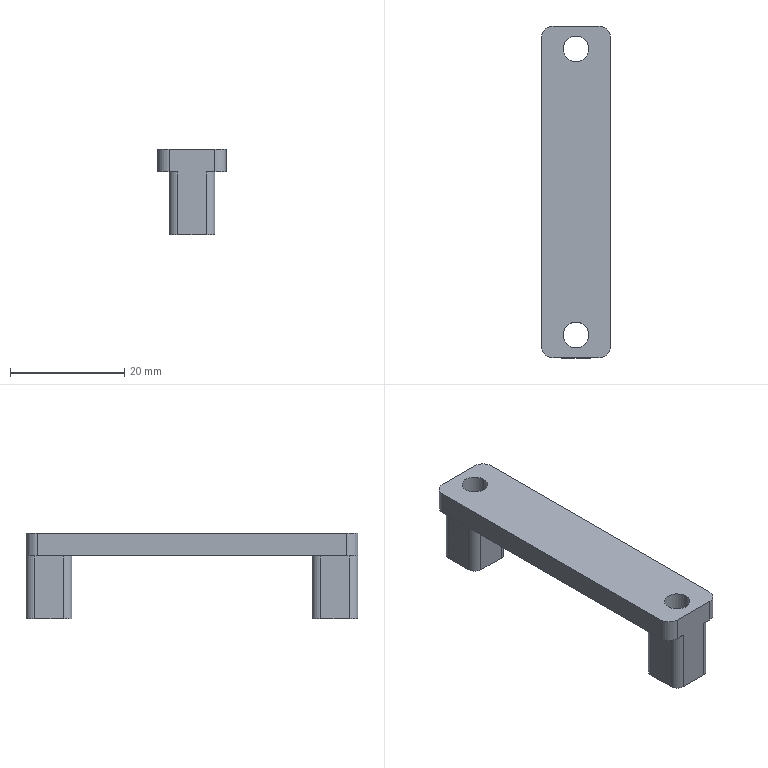Part | SolidWorks | features BaseBody 1 | 1 solid | 30 faces | box 12 x 58 x 15 mm | volume 3659 mm3 | cylinder 16 | plane 14 | commonest cylinder face diameters 3 x8 4 x4 4.5 x4
STEP:
#1=CARTESIAN_POINT('',(607.2,-29.,223.536));
#2=VERTEX_POINT('',#1);
#3=CARTESIAN_POINT('',(611.7,-29.,223.536));
#4=VERTEX_POINT('',#3);
#5=CARTESIAN_POINT('',(609.45,-29.,223.536));
#6=DIRECTION('',(0.,0.,1.));
#7=DIRECTION('',(1.,0.,0.));
#8=AXIS2_PLACEMENT_3D('',#5,#6,#7);
#9=CIRCLE('',#8,2.25);
#10=EDGE_CURVE('',#2,#4,#9,.T.);
#11=ORIENTED_EDGE('',*,*,#10,.F.);
#12=CARTESIAN_POINT('',(607.2,-29.,238.536));
#13=VERTEX_POINT('',#12);
#14=CARTESIAN_POINT('',(607.2,-29.,238.536));
#15=DIRECTION('',(0.,0.,1.));
#16=VECTOR('',#15,1000.);
#17=LINE('',#14,#16);
#18=EDGE_CURVE('',#2,#13,#17,.T.);
#19=ORIENTED_EDGE('',*,*,#18,.T.);
#20=CARTESIAN_POINT('',(611.7,-29.,238.536));
#21=VERTEX_POINT('',#20);
#22=CARTESIAN_POINT('',(609.45,-29.,238.536));
#23=DIRECTION('',(0.,0.,1.));
#24=DIRECTION('',(1.,0.,0.));
#25=AXIS2_PLACEMENT_3D('',#22,#23,#24);
#26=CIRCLE('',#25,2.25);
#27=EDGE_CURVE('',#13,#21,#26,.T.);
#28=ORIENTED_EDGE('',*,*,#27,.T.);
#29=CARTESIAN_POINT('',(611.7,-29.,238.536));
#30=DIRECTION('',(0.,0.,1.));
#31=VECTOR('',#30,1000.);
#32=LINE('',#29,#31);
#33=EDGE_CURVE('',#4,#21,#32,.T.);
#34=ORIENTED_EDGE('',*,*,#33,.F.);
#35=EDGE_LOOP('',(#11,#19,#28,#34));
#36=FACE_OUTER_BOUND('',#35,.T.);
#37=CARTESIAN_POINT('',(609.45,-29.,238.536));
#38=DIRECTION('',(0.,0.,1.));
#39=DIRECTION('',(1.,0.,0.));
#40=AXIS2_PLACEMENT_3D('',#37,#38,#39);
#41=CYLINDRICAL_SURFACE('',#40,2.25);
#42=ADVANCED_FACE('',(#36),#41,.F.);
#43=CARTESIAN_POINT('',(607.2,21.,223.536));
#44=VERTEX_POINT('',#43);
#45=CARTESIAN_POINT('',(611.7,21.,223.536));
#46=VERTEX_POINT('',#45);
#47=CARTESIAN_POINT('',(609.45,21.,223.536));
#48=DIRECTION('',(0.,0.,1.));
#49=DIRECTION('',(1.,0.,0.));
#50=AXIS2_PLACEMENT_3D('',#47,#48,#49);
#51=CIRCLE('',#50,2.25);
#52=EDGE_CURVE('',#44,#46,#51,.T.);
#53=ORIENTED_EDGE('',*,*,#52,.F.);
#54=CARTESIAN_POINT('',(607.2,21.,238.536));
#55=VERTEX_POINT('',#54);
#56=CARTESIAN_POINT('',(607.2,21.,238.536));
#57=DIRECTION('',(0.,0.,1.));
#58=VECTOR('',#57,1000.);
#59=LINE('',#56,#58);
#60=EDGE_CURVE('',#44,#55,#59,.T.);
#61=ORIENTED_EDGE('',*,*,#60,.T.);
#62=CARTESIAN_POINT('',(611.7,21.,238.536));
#63=VERTEX_POINT('',#62);
#64=CARTESIAN_POINT('',(609.45,21.,238.536));
#65=DIRECTION('',(0.,0.,1.));
#66=DIRECTION('',(1.,0.,0.));
#67=AXIS2_PLACEMENT_3D('',#64,#65,#66);
#68=CIRCLE('',#67,2.25);
#69=EDGE_CURVE('',#55,#63,#68,.T.);
#70=ORIENTED_EDGE('',*,*,#69,.T.);
#71=CARTESIAN_POINT('',(611.7,21.,238.536));
#72=DIRECTION('',(0.,0.,1.));
#73=VECTOR('',#72,1000.);
#74=LINE('',#71,#73);
#75=EDGE_CURVE('',#46,#63,#74,.T.);
#76=ORIENTED_EDGE('',*,*,#75,.F.);
#77=EDGE_LOOP('',(#53,#61,#70,#76));
#78=FACE_OUTER_BOUND('',#77,.T.);
#79=CARTESIAN_POINT('',(609.45,21.,238.536));
#80=DIRECTION('',(0.,0.,1.));
#81=DIRECTION('',(1.,0.,0.));
#82=AXIS2_PLACEMENT_3D('',#79,#80,#81);
#83=CYLINDRICAL_SURFACE('',#82,2.25);
#84=ADVANCED_FACE('',(#78),#83,.F.);
#85=CARTESIAN_POINT('',(609.45,21.,223.536));
#86=DIRECTION('',(0.,0.,1.));
#87=DIRECTION('',(1.,0.,0.));
#88=AXIS2_PLACEMENT_3D('',#85,#86,#87);
#89=CIRCLE('',#88,2.25);
#90=EDGE_CURVE('',#46,#44,#89,.T.);
#91=ORIENTED_EDGE('',*,*,#90,.T.);
#92=ORIENTED_EDGE('',*,*,#52,.T.);
#93=EDGE_LOOP('',(#91,#92));
#94=FACE_BOUND('',#93,.T.);
#95=CARTESIAN_POINT('',(611.95,25.,223.536));
#96=VERTEX_POINT('',#95);
#97=CARTESIAN_POINT('',(606.95,25.,223.536));
#98=VERTEX_POINT('',#97);
#99=CARTESIAN_POINT('',(611.95,25.,223.536));
#100=DIRECTION('',(-1.,0.,0.));
#101=VECTOR('',#100,1000.);
#102=LINE('',#99,#101);
#103=EDGE_CURVE('',#96,#98,#102,.T.);
#104=ORIENTED_EDGE('',*,*,#103,.F.);
#105=CARTESIAN_POINT('',(613.45,23.5,223.536));
#106=VERTEX_POINT('',#105);
#107=CARTESIAN_POINT('',(611.95,23.5,223.536));
#108=DIRECTION('',(0.,0.,-1.));
#109=DIRECTION('',(0.,1.,0.));
#110=AXIS2_PLACEMENT_3D('',#107,#108,#109);
#111=CIRCLE('',#110,1.5);
#112=EDGE_CURVE('',#96,#106,#111,.T.);
#113=ORIENTED_EDGE('',*,*,#112,.T.);
#114=CARTESIAN_POINT('',(613.45,18.5,223.536));
#115=VERTEX_POINT('',#114);
#116=CARTESIAN_POINT('',(613.45,18.5,223.536));
#117=DIRECTION('',(0.,1.,0.));
#118=VECTOR('',#117,1000.);
#119=LINE('',#116,#118);
#120=EDGE_CURVE('',#115,#106,#119,.T.);
#121=ORIENTED_EDGE('',*,*,#120,.F.);
#122=CARTESIAN_POINT('',(611.95,17.,223.536));
#123=VERTEX_POINT('',#122);
#124=CARTESIAN_POINT('',(611.95,18.5,223.536));
#125=DIRECTION('',(0.,0.,-1.));
#126=DIRECTION('',(1.,0.,0.));
#127=AXIS2_PLACEMENT_3D('',#124,#125,#126);
#128=CIRCLE('',#127,1.5);
#129=EDGE_CURVE('',#115,#123,#128,.T.);
#130=ORIENTED_EDGE('',*,*,#129,.T.);
#131=CARTESIAN_POINT('',(606.95,17.,223.536));
#132=VERTEX_POINT('',#131);
#133=CARTESIAN_POINT('',(606.95,17.,223.536));
#134=DIRECTION('',(1.,0.,0.));
#135=VECTOR('',#134,1000.);
#136=LINE('',#133,#135);
#137=EDGE_CURVE('',#132,#123,#136,.T.);
#138=ORIENTED_EDGE('',*,*,#137,.F.);
#139=CARTESIAN_POINT('',(605.45,18.5,223.536));
#140=VERTEX_POINT('',#139);
#141=CARTESIAN_POINT('',(606.95,18.5,223.536));
#142=DIRECTION('',(0.,0.,-1.));
#143=DIRECTION('',(0.,-1.,0.));
#144=AXIS2_PLACEMENT_3D('',#141,#142,#143);
#145=CIRCLE('',#144,1.5);
#146=EDGE_CURVE('',#132,#140,#145,.T.);
#147=ORIENTED_EDGE('',*,*,#146,.T.);
#148=CARTESIAN_POINT('',(605.45,23.5,223.536));
#149=VERTEX_POINT('',#148);
#150=CARTESIAN_POINT('',(605.45,23.5,223.536));
#151=DIRECTION('',(0.,-1.,0.));
#152=VECTOR('',#151,1000.);
#153=LINE('',#150,#152);
#154=EDGE_CURVE('',#149,#140,#153,.T.);
#155=ORIENTED_EDGE('',*,*,#154,.F.);
#156=CARTESIAN_POINT('',(606.95,23.5,223.536));
#157=DIRECTION('',(0.,0.,-1.));
#158=DIRECTION('',(-1.,0.,0.));
#159=AXIS2_PLACEMENT_3D('',#156,#157,#158);
#160=CIRCLE('',#159,1.5);
#161=EDGE_CURVE('',#149,#98,#160,.T.);
#162=ORIENTED_EDGE('',*,*,#161,.T.);
#163=EDGE_LOOP('',(#104,#113,#121,#130,#138,#147,#155,#162));
#164=FACE_OUTER_BOUND('',#163,.T.);
#165=CARTESIAN_POINT('',(615.45,-4.,223.536));
#166=DIRECTION('',(0.,0.,1.));
#167=DIRECTION('',(1.,0.,0.));
#168=AXIS2_PLACEMENT_3D('',#165,#166,#167);
#169=PLANE('',#168);
#170=ADVANCED_FACE('',(#94,#164),#169,.F.);
#171=CARTESIAN_POINT('',(609.45,-29.,223.536));
#172=DIRECTION('',(0.,0.,1.));
#173=DIRECTION('',(1.,0.,0.));
#174=AXIS2_PLACEMENT_3D('',#171,#172,#173);
#175=CIRCLE('',#174,2.25);
#176=EDGE_CURVE('',#4,#2,#175,.T.);
#177=ORIENTED_EDGE('',*,*,#176,.T.);
#178=ORIENTED_EDGE('',*,*,#10,.T.);
#179=EDGE_LOOP('',(#177,#178));
#180=FACE_BOUND('',#179,.T.);
#181=CARTESIAN_POINT('',(606.95,-33.,223.536));
#182=VERTEX_POINT('',#181);
#183=CARTESIAN_POINT('',(611.95,-33.,223.536));
#184=VERTEX_POINT('',#183);
#185=CARTESIAN_POINT('',(606.95,-33.,223.536));
#186=DIRECTION('',(1.,0.,0.));
#187=VECTOR('',#186,1000.);
#188=LINE('',#185,#187);
#189=EDGE_CURVE('',#182,#184,#188,.T.);
#190=ORIENTED_EDGE('',*,*,#189,.F.);
#191=CARTESIAN_POINT('',(605.45,-31.5,223.536));
#192=VERTEX_POINT('',#191);
#193=CARTESIAN_POINT('',(606.95,-31.5,223.536));
#194=DIRECTION('',(0.,0.,-1.));
#195=DIRECTION('',(0.,-1.,0.));
#196=AXIS2_PLACEMENT_3D('',#193,#194,#195);
#197=CIRCLE('',#196,1.5);
#198=EDGE_CURVE('',#182,#192,#197,.T.);
#199=ORIENTED_EDGE('',*,*,#198,.T.);
#200=CARTESIAN_POINT('',(605.45,-26.5,223.536));
#201=VERTEX_POINT('',#200);
#202=CARTESIAN_POINT('',(605.45,-26.5,223.536));
#203=DIRECTION('',(0.,-1.,0.));
#204=VECTOR('',#203,1000.);
#205=LINE('',#202,#204);
#206=EDGE_CURVE('',#201,#192,#205,.T.);
#207=ORIENTED_EDGE('',*,*,#206,.F.);
#208=CARTESIAN_POINT('',(606.95,-25.,223.536));
#209=VERTEX_POINT('',#208);
#210=CARTESIAN_POINT('',(606.95,-26.5,223.536));
#211=DIRECTION('',(0.,0.,-1.));
#212=DIRECTION('',(-1.,0.,0.));
#213=AXIS2_PLACEMENT_3D('',#210,#211,#212);
#214=CIRCLE('',#213,1.5);
#215=EDGE_CURVE('',#201,#209,#214,.T.);
#216=ORIENTED_EDGE('',*,*,#215,.T.);
#217=CARTESIAN_POINT('',(611.95,-25.,223.536));
#218=VERTEX_POINT('',#217);
#219=CARTESIAN_POINT('',(611.95,-25.,223.536));
#220=DIRECTION('',(-1.,0.,0.));
#221=VECTOR('',#220,1000.);
#222=LINE('',#219,#221);
#223=EDGE_CURVE('',#218,#209,#222,.T.);
#224=ORIENTED_EDGE('',*,*,#223,.F.);
#225=CARTESIAN_POINT('',(613.45,-26.5,223.536));
#226=VERTEX_POINT('',#225);
#227=CARTESIAN_POINT('',(611.95,-26.5,223.536));
#228=DIRECTION('',(0.,0.,-1.));
#229=DIRECTION('',(0.,1.,0.));
#230=AXIS2_PLACEMENT_3D('',#227,#228,#229);
#231=CIRCLE('',#230,1.5);
#232=EDGE_CURVE('',#218,#226,#231,.T.);
#233=ORIENTED_EDGE('',*,*,#232,.T.);
#234=CARTESIAN_POINT('',(613.45,-31.5,223.536));
#235=VERTEX_POINT('',#234);
#236=CARTESIAN_POINT('',(613.45,-31.5,223.536));
#237=DIRECTION('',(0.,1.,0.));
#238=VECTOR('',#237,1000.);
#239=LINE('',#236,#238);
#240=EDGE_CURVE('',#235,#226,#239,.T.);
#241=ORIENTED_EDGE('',*,*,#240,.F.);
#242=CARTESIAN_POINT('',(611.95,-31.5,223.536));
#243=DIRECTION('',(0.,0.,-1.));
#244=DIRECTION('',(1.,0.,0.));
#245=AXIS2_PLACEMENT_3D('',#242,#243,#244);
#246=CIRCLE('',#245,1.5);
#247=EDGE_CURVE('',#235,#184,#246,.T.);
#248=ORIENTED_EDGE('',*,*,#247,.T.);
#249=EDGE_LOOP('',(#190,#199,#207,#216,#224,#233,#241,#248));
#250=FACE_OUTER_BOUND('',#249,.T.);
#251=CARTESIAN_POINT('',(615.45,-4.,223.536));
#252=DIRECTION('',(0.,0.,1.));
#253=DIRECTION('',(1.,0.,0.));
#254=AXIS2_PLACEMENT_3D('',#251,#252,#253);
#255=PLANE('',#254);
#256=ADVANCED_FACE('',(#180,#250),#255,.F.);
#257=ORIENTED_EDGE('',*,*,#60,.F.);
#258=ORIENTED_EDGE('',*,*,#90,.F.);
#259=ORIENTED_EDGE('',*,*,#75,.T.);
#260=CARTESIAN_POINT('',(609.45,21.,238.536));
#261=DIRECTION('',(0.,0.,1.));
#262=DIRECTION('',(1.,0.,0.));
#263=AXIS2_PLACEMENT_3D('',#260,#261,#262);
#264=CIRCLE('',#263,2.25);
#265=EDGE_CURVE('',#63,#55,#264,.T.);
#266=ORIENTED_EDGE('',*,*,#265,.T.);
#267=EDGE_LOOP('',(#257,#258,#259,#266));
#268=FACE_OUTER_BOUND('',#267,.T.);
#269=CARTESIAN_POINT('',(609.45,21.,238.536));
#270=DIRECTION('',(0.,0.,1.));
#271=DIRECTION('',(1.,0.,0.));
#272=AXIS2_PLACEMENT_3D('',#269,#270,#271);
#273=CYLINDRICAL_SURFACE('',#272,2.25);
#274=ADVANCED_FACE('',(#268),#273,.F.);
#275=ORIENTED_EDGE('',*,*,#265,.F.);
#276=ORIENTED_EDGE('',*,*,#69,.F.);
#277=EDGE_LOOP('',(#275,#276));
#278=FACE_BOUND('',#277,.T.);
#279=CARTESIAN_POINT('',(609.45,-29.,238.536));
#280=DIRECTION('',(0.,0.,1.));
#281=DIRECTION('',(1.,0.,0.));
#282=AXIS2_PLACEMENT_3D('',#279,#280,#281);
#283=CIRCLE('',#282,2.25);
#284=EDGE_CURVE('',#21,#13,#283,.T.);
#285=ORIENTED_EDGE('',*,*,#284,.F.);
#286=ORIENTED_EDGE('',*,*,#27,.F.);
#287=EDGE_LOOP('',(#285,#286));
#288=FACE_BOUND('',#287,.T.);
#289=CARTESIAN_POINT('',(605.45,25.,238.536));
#290=VERTEX_POINT('',#289);
#291=CARTESIAN_POINT('',(613.45,25.,238.536));
#292=VERTEX_POINT('',#291);
#293=CARTESIAN_POINT('',(605.45,25.,238.536));
#294=DIRECTION('',(1.,0.,0.));
#295=VECTOR('',#294,1000.);
#296=LINE('',#293,#295);
#297=EDGE_CURVE('',#290,#292,#296,.T.);
#298=ORIENTED_EDGE('',*,*,#297,.F.);
#299=CARTESIAN_POINT('',(603.45,23.,238.536));
#300=VERTEX_POINT('',#299);
#301=CARTESIAN_POINT('',(605.45,23.,238.536));
#302=DIRECTION('',(0.,0.,1.));
#303=DIRECTION('',(0.,1.,0.));
#304=AXIS2_PLACEMENT_3D('',#301,#302,#303);
#305=CIRCLE('',#304,2.);
#306=EDGE_CURVE('',#290,#300,#305,.T.);
#307=ORIENTED_EDGE('',*,*,#306,.T.);
#308=CARTESIAN_POINT('',(603.45,-31.,238.536));
#309=VERTEX_POINT('',#308);
#310=CARTESIAN_POINT('',(603.45,23.,238.536));
#311=DIRECTION('',(0.,-1.,0.));
#312=VECTOR('',#311,1000.);
#313=LINE('',#310,#312);
#314=EDGE_CURVE('',#300,#309,#313,.T.);
#315=ORIENTED_EDGE('',*,*,#314,.T.);
#316=CARTESIAN_POINT('',(605.45,-33.,238.536));
#317=VERTEX_POINT('',#316);
#318=CARTESIAN_POINT('',(605.45,-31.,238.536));
#319=DIRECTION('',(0.,0.,1.));
#320=DIRECTION('',(-1.,0.,0.));
#321=AXIS2_PLACEMENT_3D('',#318,#319,#320);
#322=CIRCLE('',#321,2.);
#323=EDGE_CURVE('',#309,#317,#322,.T.);
#324=ORIENTED_EDGE('',*,*,#323,.T.);
#325=CARTESIAN_POINT('',(613.45,-33.,238.536));
#326=VERTEX_POINT('',#325);
#327=CARTESIAN_POINT('',(613.45,-33.,238.536));
#328=DIRECTION('',(-1.,0.,0.));
#329=VECTOR('',#328,1000.);
#330=LINE('',#327,#329);
#331=EDGE_CURVE('',#326,#317,#330,.T.);
#332=ORIENTED_EDGE('',*,*,#331,.F.);
#333=CARTESIAN_POINT('',(615.45,-31.,238.536));
#334=VERTEX_POINT('',#333);
#335=CARTESIAN_POINT('',(613.45,-31.,238.536));
#336=DIRECTION('',(0.,0.,1.));
#337=DIRECTION('',(0.,-1.,0.));
#338=AXIS2_PLACEMENT_3D('',#335,#336,#337);
#339=CIRCLE('',#338,2.);
#340=EDGE_CURVE('',#326,#334,#339,.T.);
#341=ORIENTED_EDGE('',*,*,#340,.T.);
#342=CARTESIAN_POINT('',(615.45,23.,238.536));
#343=VERTEX_POINT('',#342);
#344=CARTESIAN_POINT('',(615.45,-31.,238.536));
#345=DIRECTION('',(0.,1.,0.));
#346=VECTOR('',#345,1000.);
#347=LINE('',#344,#346);
#348=EDGE_CURVE('',#334,#343,#347,.T.);
#349=ORIENTED_EDGE('',*,*,#348,.T.);
#350=CARTESIAN_POINT('',(613.45,23.,238.536));
#351=DIRECTION('',(0.,0.,1.));
#352=DIRECTION('',(1.,0.,0.));
#353=AXIS2_PLACEMENT_3D('',#350,#351,#352);
#354=CIRCLE('',#353,2.);
#355=EDGE_CURVE('',#343,#292,#354,.T.);
#356=ORIENTED_EDGE('',*,*,#355,.T.);
#357=EDGE_LOOP('',(#298,#307,#315,#324,#332,#341,#349,#356));
#358=FACE_OUTER_BOUND('',#357,.T.);
#359=CARTESIAN_POINT('',(615.45,-4.,238.536));
#360=DIRECTION('',(0.,0.,1.));
#361=DIRECTION('',(1.,0.,0.));
#362=AXIS2_PLACEMENT_3D('',#359,#360,#361);
#363=PLANE('',#362);
#364=ADVANCED_FACE('',(#278,#288,#358),#363,.T.);
#365=CARTESIAN_POINT('',(613.45,25.,234.536));
#366=VERTEX_POINT('',#365);
#367=CARTESIAN_POINT('',(613.45,25.,238.536));
#368=DIRECTION('',(0.,0.,-1.));
#369=VECTOR('',#368,1000.);
#370=LINE('',#367,#369);
#371=EDGE_CURVE('',#292,#366,#370,.T.);
#372=ORIENTED_EDGE('',*,*,#371,.F.);
#373=ORIENTED_EDGE('',*,*,#355,.F.);
#374=CARTESIAN_POINT('',(615.45,23.,234.536));
#375=VERTEX_POINT('',#374);
#376=CARTESIAN_POINT('',(615.45,23.,238.536));
#377=DIRECTION('',(0.,0.,-1.));
#378=VECTOR('',#377,1000.);
#379=LINE('',#376,#378);
#380=EDGE_CURVE('',#343,#375,#379,.T.);
#381=ORIENTED_EDGE('',*,*,#380,.T.);
#382=CARTESIAN_POINT('',(613.45,23.,234.536));
#383=DIRECTION('',(0.,0.,-1.));
#384=DIRECTION('',(0.,1.,0.));
#385=AXIS2_PLACEMENT_3D('',#382,#383,#384);
#386=CIRCLE('',#385,2.);
#387=EDGE_CURVE('',#366,#375,#386,.T.);
#388=ORIENTED_EDGE('',*,*,#387,.F.);
#389=EDGE_LOOP('',(#372,#373,#381,#388));
#390=FACE_OUTER_BOUND('',#389,.T.);
#391=CARTESIAN_POINT('',(613.45,23.,258.09));
#392=DIRECTION('',(0.,0.,-1.));
#393=DIRECTION('',(0.,-1.,0.));
#394=AXIS2_PLACEMENT_3D('',#391,#392,#393);
#395=CYLINDRICAL_SURFACE('',#394,2.);
#396=ADVANCED_FACE('',(#390),#395,.T.);
#397=CARTESIAN_POINT('',(615.45,-31.,234.536));
#398=VERTEX_POINT('',#397);
#399=CARTESIAN_POINT('',(615.45,23.,234.536));
#400=DIRECTION('',(0.,-1.,0.));
#401=VECTOR('',#400,1000.);
#402=LINE('',#399,#401);
#403=EDGE_CURVE('',#375,#398,#402,.T.);
#404=ORIENTED_EDGE('',*,*,#403,.T.);
#405=CARTESIAN_POINT('',(613.45,-33.,234.536));
#406=VERTEX_POINT('',#405);
#407=CARTESIAN_POINT('',(613.45,-31.,234.536));
#408=DIRECTION('',(0.,0.,-1.));
#409=DIRECTION('',(1.,0.,0.));
#410=AXIS2_PLACEMENT_3D('',#407,#408,#409);
#411=CIRCLE('',#410,2.);
#412=EDGE_CURVE('',#398,#406,#411,.T.);
#413=ORIENTED_EDGE('',*,*,#412,.T.);
#414=CARTESIAN_POINT('',(611.95,-33.,234.536));
#415=VERTEX_POINT('',#414);
#416=CARTESIAN_POINT('',(611.95,-33.,234.536));
#417=DIRECTION('',(-1.,0.,0.));
#418=VECTOR('',#417,1000.);
#419=LINE('',#416,#418);
#420=EDGE_CURVE('',#406,#415,#419,.T.);
#421=ORIENTED_EDGE('',*,*,#420,.T.);
#422=CARTESIAN_POINT('',(613.45,-31.5,234.536));
#423=VERTEX_POINT('',#422);
#424=CARTESIAN_POINT('',(611.95,-31.5,234.536));
#425=DIRECTION('',(0.,0.,1.));
#426=DIRECTION('',(0.,-1.,0.));
#427=AXIS2_PLACEMENT_3D('',#424,#425,#426);
#428=CIRCLE('',#427,1.5);
#429=EDGE_CURVE('',#415,#423,#428,.T.);
#430=ORIENTED_EDGE('',*,*,#429,.T.);
#431=CARTESIAN_POINT('',(613.45,-26.5,234.536));
#432=VERTEX_POINT('',#431);
#433=CARTESIAN_POINT('',(613.45,-26.5,234.536));
#434=DIRECTION('',(0.,-1.,0.));
#435=VECTOR('',#434,1000.);
#436=LINE('',#433,#435);
#437=EDGE_CURVE('',#432,#423,#436,.T.);
#438=ORIENTED_EDGE('',*,*,#437,.F.);
#439=CARTESIAN_POINT('',(611.95,-25.,234.536));
#440=VERTEX_POINT('',#439);
#441=CARTESIAN_POINT('',(611.95,-26.5,234.536));
#442=DIRECTION('',(0.,0.,1.));
#443=DIRECTION('',(1.,0.,0.));
#444=AXIS2_PLACEMENT_3D('',#441,#442,#443);
#445=CIRCLE('',#444,1.5);
#446=EDGE_CURVE('',#432,#440,#445,.T.);
#447=ORIENTED_EDGE('',*,*,#446,.T.);
#448=CARTESIAN_POINT('',(606.95,-25.,234.536));
#449=VERTEX_POINT('',#448);
#450=CARTESIAN_POINT('',(606.95,-25.,234.536));
#451=DIRECTION('',(1.,0.,0.));
#452=VECTOR('',#451,1000.);
#453=LINE('',#450,#452);
#454=EDGE_CURVE('',#449,#440,#453,.T.);
#455=ORIENTED_EDGE('',*,*,#454,.F.);
#456=CARTESIAN_POINT('',(605.45,-26.5,234.536));
#457=VERTEX_POINT('',#456);
#458=CARTESIAN_POINT('',(606.95,-26.5,234.536));
#459=DIRECTION('',(0.,0.,1.));
#460=DIRECTION('',(0.,1.,0.));
#461=AXIS2_PLACEMENT_3D('',#458,#459,#460);
#462=CIRCLE('',#461,1.5);
#463=EDGE_CURVE('',#449,#457,#462,.T.);
#464=ORIENTED_EDGE('',*,*,#463,.T.);
#465=CARTESIAN_POINT('',(605.45,-31.5,234.536));
#466=VERTEX_POINT('',#465);
#467=CARTESIAN_POINT('',(605.45,-31.5,234.536));
#468=DIRECTION('',(0.,1.,0.));
#469=VECTOR('',#468,1000.);
#470=LINE('',#467,#469);
#471=EDGE_CURVE('',#466,#457,#470,.T.);
#472=ORIENTED_EDGE('',*,*,#471,.F.);
#473=CARTESIAN_POINT('',(606.95,-33.,234.536));
#474=VERTEX_POINT('',#473);
#475=CARTESIAN_POINT('',(606.95,-31.5,234.536));
#476=DIRECTION('',(0.,0.,1.));
#477=DIRECTION('',(-1.,0.,0.));
#478=AXIS2_PLACEMENT_3D('',#475,#476,#477);
#479=CIRCLE('',#478,1.5);
#480=EDGE_CURVE('',#466,#474,#479,.T.);
#481=ORIENTED_EDGE('',*,*,#480,.T.);
#482=CARTESIAN_POINT('',(605.45,-33.,234.536));
#483=VERTEX_POINT('',#482);
#484=CARTESIAN_POINT('',(606.95,-33.,234.536));
#485=DIRECTION('',(1.,0.,0.));
#486=VECTOR('',#485,1000.);
#487=LINE('',#484,#486);
#488=EDGE_CURVE('',#483,#474,#487,.T.);
#489=ORIENTED_EDGE('',*,*,#488,.F.);
#490=CARTESIAN_POINT('',(603.45,-31.,234.536));
#491=VERTEX_POINT('',#490);
#492=CARTESIAN_POINT('',(605.45,-31.,234.536));
#493=DIRECTION('',(0.,0.,-1.));
#494=DIRECTION('',(0.,-1.,0.));
#495=AXIS2_PLACEMENT_3D('',#492,#493,#494);
#496=CIRCLE('',#495,2.);
#497=EDGE_CURVE('',#483,#491,#496,.T.);
#498=ORIENTED_EDGE('',*,*,#497,.T.);
#499=CARTESIAN_POINT('',(603.45,23.,234.536));
#500=VERTEX_POINT('',#499);
#501=CARTESIAN_POINT('',(603.45,-31.,234.536));
#502=DIRECTION('',(0.,1.,0.));
#503=VECTOR('',#502,1000.);
#504=LINE('',#501,#503);
#505=EDGE_CURVE('',#491,#500,#504,.T.);
#506=ORIENTED_EDGE('',*,*,#505,.T.);
#507=CARTESIAN_POINT('',(605.45,25.,234.536));
#508=VERTEX_POINT('',#507);
#509=CARTESIAN_POINT('',(605.45,23.,234.536));
#510=DIRECTION('',(0.,0.,-1.));
#511=DIRECTION('',(-1.,0.,0.));
#512=AXIS2_PLACEMENT_3D('',#509,#510,#511);
#513=CIRCLE('',#512,2.);
#514=EDGE_CURVE('',#500,#508,#513,.T.);
#515=ORIENTED_EDGE('',*,*,#514,.T.);
#516=CARTESIAN_POINT('',(606.95,25.,234.536));
#517=VERTEX_POINT('',#516);
#518=CARTESIAN_POINT('',(606.95,25.,234.536));
#519=DIRECTION('',(-1.,0.,0.));
#520=VECTOR('',#519,1000.);
#521=LINE('',#518,#520);
#522=EDGE_CURVE('',#517,#508,#521,.T.);
#523=ORIENTED_EDGE('',*,*,#522,.F.);
#524=CARTESIAN_POINT('',(605.45,23.5,234.536));
#525=VERTEX_POINT('',#524);
#526=CARTESIAN_POINT('',(606.95,23.5,234.536));
#527=DIRECTION('',(0.,0.,1.));
#528=DIRECTION('',(0.,1.,0.));
#529=AXIS2_PLACEMENT_3D('',#526,#527,#528);
#530=CIRCLE('',#529,1.5);
#531=EDGE_CURVE('',#517,#525,#530,.T.);
#532=ORIENTED_EDGE('',*,*,#531,.T.);
#533=CARTESIAN_POINT('',(605.45,18.5,234.536));
#534=VERTEX_POINT('',#533);
#535=CARTESIAN_POINT('',(605.45,18.5,234.536));
#536=DIRECTION('',(0.,1.,0.));
#537=VECTOR('',#536,1000.);
#538=LINE('',#535,#537);
#539=EDGE_CURVE('',#534,#525,#538,.T.);
#540=ORIENTED_EDGE('',*,*,#539,.F.);
#541=CARTESIAN_POINT('',(606.95,17.,234.536));
#542=VERTEX_POINT('',#541);
#543=CARTESIAN_POINT('',(606.95,18.5,234.536));
#544=DIRECTION('',(0.,0.,1.));
#545=DIRECTION('',(-1.,0.,0.));
#546=AXIS2_PLACEMENT_3D('',#543,#544,#545);
#547=CIRCLE('',#546,1.5);
#548=EDGE_CURVE('',#534,#542,#547,.T.);
#549=ORIENTED_EDGE('',*,*,#548,.T.);
#550=CARTESIAN_POINT('',(611.95,17.,234.536));
#551=VERTEX_POINT('',#550);
#552=CARTESIAN_POINT('',(611.95,17.,234.536));
#553=DIRECTION('',(-1.,0.,0.));
#554=VECTOR('',#553,1000.);
#555=LINE('',#552,#554);
#556=EDGE_CURVE('',#551,#542,#555,.T.);
#557=ORIENTED_EDGE('',*,*,#556,.F.);
#558=CARTESIAN_POINT('',(613.45,18.5,234.536));
#559=VERTEX_POINT('',#558);
#560=CARTESIAN_POINT('',(611.95,18.5,234.536));
#561=DIRECTION('',(0.,0.,1.));
#562=DIRECTION('',(0.,-1.,0.));
#563=AXIS2_PLACEMENT_3D('',#560,#561,#562);
#564=CIRCLE('',#563,1.5);
#565=EDGE_CURVE('',#551,#559,#564,.T.);
#566=ORIENTED_EDGE('',*,*,#565,.T.);
#567=CARTESIAN_POINT('',(613.45,23.5,234.536));
#568=VERTEX_POINT('',#567);
#569=CARTESIAN_POINT('',(613.45,23.5,234.536));
#570=DIRECTION('',(0.,-1.,0.));
#571=VECTOR('',#570,1000.);
#572=LINE('',#569,#571);
#573=EDGE_CURVE('',#568,#559,#572,.T.);
#574=ORIENTED_EDGE('',*,*,#573,.F.);
#575=CARTESIAN_POINT('',(611.95,25.,234.536));
#576=VERTEX_POINT('',#575);
#577=CARTESIAN_POINT('',(611.95,23.5,234.536));
#578=DIRECTION('',(0.,0.,1.));
#579=DIRECTION('',(1.,0.,0.));
#580=AXIS2_PLACEMENT_3D('',#577,#578,#579);
#581=CIRCLE('',#580,1.5);
#582=EDGE_CURVE('',#568,#576,#581,.T.);
#583=ORIENTED_EDGE('',*,*,#582,.T.);
#584=CARTESIAN_POINT('',(611.95,25.,234.536));
#585=DIRECTION('',(1.,0.,0.));
#586=VECTOR('',#585,1000.);
#587=LINE('',#584,#586);
#588=EDGE_CURVE('',#576,#366,#587,.T.);
#589=ORIENTED_EDGE('',*,*,#588,.T.);
#590=ORIENTED_EDGE('',*,*,#387,.T.);
#591=EDGE_LOOP('',(#404,#413,#421,#430,#438,#447,#455,#464,#472,#481,#489,#498,#506,#515,#523,#532,#540,#549,#557,#566,#574,#583,#589,#590));
#592=FACE_OUTER_BOUND('',#591,.T.);
#593=CARTESIAN_POINT('',(91.046,-4.,234.536));
#594=DIRECTION('',(0.,0.,1.));
#595=DIRECTION('',(1.,0.,0.));
#596=AXIS2_PLACEMENT_3D('',#593,#594,#595);
#597=PLANE('',#596);
#598=ADVANCED_FACE('',(#592),#597,.F.);
#599=ORIENTED_EDGE('',*,*,#522,.T.);
#600=CARTESIAN_POINT('',(605.45,25.,238.536));
#601=DIRECTION('',(0.,0.,-1.));
#602=VECTOR('',#601,1000.);
#603=LINE('',#600,#602);
#604=EDGE_CURVE('',#290,#508,#603,.T.);
#605=ORIENTED_EDGE('',*,*,#604,.F.);
#606=ORIENTED_EDGE('',*,*,#297,.T.);
#607=ORIENTED_EDGE('',*,*,#371,.T.);
#608=ORIENTED_EDGE('',*,*,#588,.F.);
#609=CARTESIAN_POINT('',(611.95,25.,223.536));
#610=DIRECTION('',(0.,0.,1.));
#611=VECTOR('',#610,1000.);
#612=LINE('',#609,#611);
#613=EDGE_CURVE('',#96,#576,#612,.T.);
#614=ORIENTED_EDGE('',*,*,#613,.F.);
#615=ORIENTED_EDGE('',*,*,#103,.T.);
#616=CARTESIAN_POINT('',(606.95,25.,223.536));
#617=DIRECTION('',(0.,0.,1.));
#618=VECTOR('',#617,1000.);
#619=LINE('',#616,#618);
#620=EDGE_CURVE('',#98,#517,#619,.T.);
#621=ORIENTED_EDGE('',*,*,#620,.T.);
#622=EDGE_LOOP('',(#599,#605,#606,#607,#608,#614,#615,#621));
#623=FACE_OUTER_BOUND('',#622,.T.);
#624=CARTESIAN_POINT('',(615.45,25.,238.536));
#625=DIRECTION('',(0.,1.,0.));
#626=DIRECTION('',(1.,0.,0.));
#627=AXIS2_PLACEMENT_3D('',#624,#625,#626);
#628=PLANE('',#627);
#629=ADVANCED_FACE('',(#623),#628,.T.);
#630=ORIENTED_EDGE('',*,*,#531,.F.);
#631=ORIENTED_EDGE('',*,*,#620,.F.);
#632=ORIENTED_EDGE('',*,*,#161,.F.);
#633=CARTESIAN_POINT('',(605.45,23.5,223.536));
#634=DIRECTION('',(0.,0.,1.));
#635=VECTOR('',#634,1000.);
#636=LINE('',#633,#635);
#637=EDGE_CURVE('',#149,#525,#636,.T.);
#638=ORIENTED_EDGE('',*,*,#637,.T.);
#639=EDGE_LOOP('',(#630,#631,#632,#638));
#640=FACE_OUTER_BOUND('',#639,.T.);
#641=CARTESIAN_POINT('',(606.95,23.5,203.982));
#642=DIRECTION('',(0.,0.,1.));
#643=DIRECTION('',(0.,-1.,0.));
#644=AXIS2_PLACEMENT_3D('',#641,#642,#643);
#645=CYLINDRICAL_SURFACE('',#644,1.5);
#646=ADVANCED_FACE('',(#640),#645,.T.);
#647=ORIENTED_EDGE('',*,*,#154,.T.);
#648=CARTESIAN_POINT('',(605.45,18.5,223.536));
#649=DIRECTION('',(0.,0.,1.));
#650=VECTOR('',#649,1000.);
#651=LINE('',#648,#650);
#652=EDGE_CURVE('',#140,#534,#651,.T.);
#653=ORIENTED_EDGE('',*,*,#652,.T.);
#654=ORIENTED_EDGE('',*,*,#539,.T.);
#655=ORIENTED_EDGE('',*,*,#637,.F.);
#656=EDGE_LOOP('',(#647,#653,#654,#655));
#657=FACE_OUTER_BOUND('',#656,.T.);
#658=CARTESIAN_POINT('',(605.45,17.,223.536));
#659=DIRECTION('',(-1.,0.,0.));
#660=DIRECTION('',(0.,0.,1.));
#661=AXIS2_PLACEMENT_3D('',#658,#659,#660);
#662=PLANE('',#661);
#663=ADVANCED_FACE('',(#657),#662,.T.);
#664=ORIENTED_EDGE('',*,*,#548,.F.);
#665=ORIENTED_EDGE('',*,*,#652,.F.);
#666=ORIENTED_EDGE('',*,*,#146,.F.);
#667=CARTESIAN_POINT('',(606.95,17.,223.536));
#668=DIRECTION('',(0.,0.,1.));
#669=VECTOR('',#668,1000.);
#670=LINE('',#667,#669);
#671=EDGE_CURVE('',#132,#542,#670,.T.);
#672=ORIENTED_EDGE('',*,*,#671,.T.);
#673=EDGE_LOOP('',(#664,#665,#666,#672));
#674=FACE_OUTER_BOUND('',#673,.T.);
#675=CARTESIAN_POINT('',(606.95,18.5,203.982));
#676=DIRECTION('',(0.,0.,1.));
#677=DIRECTION('',(1.,0.,0.));
#678=AXIS2_PLACEMENT_3D('',#675,#676,#677);
#679=CYLINDRICAL_SURFACE('',#678,1.5);
#680=ADVANCED_FACE('',(#674),#679,.T.);
#681=ORIENTED_EDGE('',*,*,#556,.T.);
#682=ORIENTED_EDGE('',*,*,#671,.F.);
#683=ORIENTED_EDGE('',*,*,#137,.T.);
#684=CARTESIAN_POINT('',(611.95,17.,223.536));
#685=DIRECTION('',(0.,0.,1.));
#686=VECTOR('',#685,1000.);
#687=LINE('',#684,#686);
#688=EDGE_CURVE('',#123,#551,#687,.T.);
#689=ORIENTED_EDGE('',*,*,#688,.T.);
#690=EDGE_LOOP('',(#681,#682,#683,#689));
#691=FACE_OUTER_BOUND('',#690,.T.);
#692=CARTESIAN_POINT('',(613.45,17.,223.536));
#693=DIRECTION('',(0.,-1.,0.));
#694=DIRECTION('',(0.,0.,-1.));
#695=AXIS2_PLACEMENT_3D('',#692,#693,#694);
#696=PLANE('',#695);
#697=ADVANCED_FACE('',(#691),#696,.T.);
#698=ORIENTED_EDGE('',*,*,#565,.F.);
#699=ORIENTED_EDGE('',*,*,#688,.F.);
#700=ORIENTED_EDGE('',*,*,#129,.F.);
#701=CARTESIAN_POINT('',(613.45,18.5,223.536));
#702=DIRECTION('',(0.,0.,1.));
#703=VECTOR('',#702,1000.);
#704=LINE('',#701,#703);
#705=EDGE_CURVE('',#115,#559,#704,.T.);
#706=ORIENTED_EDGE('',*,*,#705,.T.);
#707=EDGE_LOOP('',(#698,#699,#700,#706));
#708=FACE_OUTER_BOUND('',#707,.T.);
#709=CARTESIAN_POINT('',(611.95,18.5,203.982));
#710=DIRECTION('',(0.,0.,1.));
#711=DIRECTION('',(0.,1.,0.));
#712=AXIS2_PLACEMENT_3D('',#709,#710,#711);
#713=CYLINDRICAL_SURFACE('',#712,1.5);
#714=ADVANCED_FACE('',(#708),#713,.T.);
#715=ORIENTED_EDGE('',*,*,#573,.T.);
#716=ORIENTED_EDGE('',*,*,#705,.F.);
#717=ORIENTED_EDGE('',*,*,#120,.T.);
#718=CARTESIAN_POINT('',(613.45,23.5,223.536));
#719=DIRECTION('',(0.,0.,1.));
#720=VECTOR('',#719,1000.);
#721=LINE('',#718,#720);
#722=EDGE_CURVE('',#106,#568,#721,.T.);
#723=ORIENTED_EDGE('',*,*,#722,.T.);
#724=EDGE_LOOP('',(#715,#716,#717,#723));
#725=FACE_OUTER_BOUND('',#724,.T.);
#726=CARTESIAN_POINT('',(613.45,25.,223.536));
#727=DIRECTION('',(1.,0.,0.));
#728=DIRECTION('',(0.,1.,0.));
#729=AXIS2_PLACEMENT_3D('',#726,#727,#728);
#730=PLANE('',#729);
#731=ADVANCED_FACE('',(#725),#730,.T.);
#732=ORIENTED_EDGE('',*,*,#582,.F.);
#733=ORIENTED_EDGE('',*,*,#722,.F.);
#734=ORIENTED_EDGE('',*,*,#112,.F.);
#735=ORIENTED_EDGE('',*,*,#613,.T.);
#736=EDGE_LOOP('',(#732,#733,#734,#735));
#737=FACE_OUTER_BOUND('',#736,.T.);
#738=CARTESIAN_POINT('',(611.95,23.5,203.982));
#739=DIRECTION('',(0.,0.,1.));
#740=DIRECTION('',(-1.,0.,0.));
#741=AXIS2_PLACEMENT_3D('',#738,#739,#740);
#742=CYLINDRICAL_SURFACE('',#741,1.5);
#743=ADVANCED_FACE('',(#737),#742,.T.);
#744=CARTESIAN_POINT('',(603.45,23.,238.536));
#745=DIRECTION('',(0.,0.,-1.));
#746=VECTOR('',#745,1000.);
#747=LINE('',#744,#746);
#748=EDGE_CURVE('',#300,#500,#747,.T.);
#749=ORIENTED_EDGE('',*,*,#748,.F.);
#750=ORIENTED_EDGE('',*,*,#306,.F.);
#751=ORIENTED_EDGE('',*,*,#604,.T.);
#752=ORIENTED_EDGE('',*,*,#514,.F.);
#753=EDGE_LOOP('',(#749,#750,#751,#752));
#754=FACE_OUTER_BOUND('',#753,.T.);
#755=CARTESIAN_POINT('',(605.45,23.,258.09));
#756=DIRECTION('',(0.,0.,-1.));
#757=DIRECTION('',(1.,0.,0.));
#758=AXIS2_PLACEMENT_3D('',#755,#756,#757);
#759=CYLINDRICAL_SURFACE('',#758,2.);
#760=ADVANCED_FACE('',(#754),#759,.T.);
#761=ORIENTED_EDGE('',*,*,#505,.F.);
#762=CARTESIAN_POINT('',(603.45,-31.,238.536));
#763=DIRECTION('',(0.,0.,-1.));
#764=VECTOR('',#763,1000.);
#765=LINE('',#762,#764);
#766=EDGE_CURVE('',#309,#491,#765,.T.);
#767=ORIENTED_EDGE('',*,*,#766,.F.);
#768=ORIENTED_EDGE('',*,*,#314,.F.);
#769=ORIENTED_EDGE('',*,*,#748,.T.);
#770=EDGE_LOOP('',(#761,#767,#768,#769));
#771=FACE_OUTER_BOUND('',#770,.T.);
#772=CARTESIAN_POINT('',(603.45,25.,238.536));
#773=DIRECTION('',(-1.,0.,0.));
#774=DIRECTION('',(0.,0.,1.));
#775=AXIS2_PLACEMENT_3D('',#772,#773,#774);
#776=PLANE('',#775);
#777=ADVANCED_FACE('',(#771),#776,.T.);
#778=CARTESIAN_POINT('',(605.45,-33.,238.536));
#779=DIRECTION('',(0.,0.,-1.));
#780=VECTOR('',#779,1000.);
#781=LINE('',#778,#780);
#782=EDGE_CURVE('',#317,#483,#781,.T.);
#783=ORIENTED_EDGE('',*,*,#782,.F.);
#784=ORIENTED_EDGE('',*,*,#323,.F.);
#785=ORIENTED_EDGE('',*,*,#766,.T.);
#786=ORIENTED_EDGE('',*,*,#497,.F.);
#787=EDGE_LOOP('',(#783,#784,#785,#786));
#788=FACE_OUTER_BOUND('',#787,.T.);
#789=CARTESIAN_POINT('',(605.45,-31.,258.09));
#790=DIRECTION('',(0.,0.,-1.));
#791=DIRECTION('',(0.,1.,0.));
#792=AXIS2_PLACEMENT_3D('',#789,#790,#791);
#793=CYLINDRICAL_SURFACE('',#792,2.);
#794=ADVANCED_FACE('',(#788),#793,.T.);
#795=ORIENTED_EDGE('',*,*,#420,.F.);
#796=CARTESIAN_POINT('',(613.45,-33.,238.536));
#797=DIRECTION('',(0.,0.,-1.));
#798=VECTOR('',#797,1000.);
#799=LINE('',#796,#798);
#800=EDGE_CURVE('',#326,#406,#799,.T.);
#801=ORIENTED_EDGE('',*,*,#800,.F.);
#802=ORIENTED_EDGE('',*,*,#331,.T.);
#803=ORIENTED_EDGE('',*,*,#782,.T.);
#804=ORIENTED_EDGE('',*,*,#488,.T.);
#805=CARTESIAN_POINT('',(606.95,-33.,223.536));
#806=DIRECTION('',(0.,0.,1.));
#807=VECTOR('',#806,1000.);
#808=LINE('',#805,#807);
#809=EDGE_CURVE('',#182,#474,#808,.T.);
#810=ORIENTED_EDGE('',*,*,#809,.F.);
#811=ORIENTED_EDGE('',*,*,#189,.T.);
#812=CARTESIAN_POINT('',(611.95,-33.,223.536));
#813=DIRECTION('',(0.,0.,1.));
#814=VECTOR('',#813,1000.);
#815=LINE('',#812,#814);
#816=EDGE_CURVE('',#184,#415,#815,.T.);
#817=ORIENTED_EDGE('',*,*,#816,.T.);
#818=EDGE_LOOP('',(#795,#801,#802,#803,#804,#810,#811,#817));
#819=FACE_OUTER_BOUND('',#818,.T.);
#820=CARTESIAN_POINT('',(603.45,-33.,238.536));
#821=DIRECTION('',(0.,-1.,0.));
#822=DIRECTION('',(0.,0.,-1.));
#823=AXIS2_PLACEMENT_3D('',#820,#821,#822);
#824=PLANE('',#823);
#825=ADVANCED_FACE('',(#819),#824,.T.);
#826=ORIENTED_EDGE('',*,*,#429,.F.);
#827=ORIENTED_EDGE('',*,*,#816,.F.);
#828=ORIENTED_EDGE('',*,*,#247,.F.);
#829=CARTESIAN_POINT('',(613.45,-31.5,223.536));
#830=DIRECTION('',(0.,0.,1.));
#831=VECTOR('',#830,1000.);
#832=LINE('',#829,#831);
#833=EDGE_CURVE('',#235,#423,#832,.T.);
#834=ORIENTED_EDGE('',*,*,#833,.T.);
#835=EDGE_LOOP('',(#826,#827,#828,#834));
#836=FACE_OUTER_BOUND('',#835,.T.);
#837=CARTESIAN_POINT('',(611.95,-31.5,203.982));
#838=DIRECTION('',(0.,0.,1.));
#839=DIRECTION('',(0.,1.,0.));
#840=AXIS2_PLACEMENT_3D('',#837,#838,#839);
#841=CYLINDRICAL_SURFACE('',#840,1.5);
#842=ADVANCED_FACE('',(#836),#841,.T.);
#843=ORIENTED_EDGE('',*,*,#240,.T.);
#844=CARTESIAN_POINT('',(613.45,-26.5,223.536));
#845=DIRECTION('',(0.,0.,1.));
#846=VECTOR('',#845,1000.);
#847=LINE('',#844,#846);
#848=EDGE_CURVE('',#226,#432,#847,.T.);
#849=ORIENTED_EDGE('',*,*,#848,.T.);
#850=ORIENTED_EDGE('',*,*,#437,.T.);
#851=ORIENTED_EDGE('',*,*,#833,.F.);
#852=EDGE_LOOP('',(#843,#849,#850,#851));
#853=FACE_OUTER_BOUND('',#852,.T.);
#854=CARTESIAN_POINT('',(613.45,-25.,223.536));
#855=DIRECTION('',(1.,0.,0.));
#856=DIRECTION('',(0.,1.,0.));
#857=AXIS2_PLACEMENT_3D('',#854,#855,#856);
#858=PLANE('',#857);
#859=ADVANCED_FACE('',(#853),#858,.T.);
#860=ORIENTED_EDGE('',*,*,#446,.F.);
#861=ORIENTED_EDGE('',*,*,#848,.F.);
#862=ORIENTED_EDGE('',*,*,#232,.F.);
#863=CARTESIAN_POINT('',(611.95,-25.,223.536));
#864=DIRECTION('',(0.,0.,1.));
#865=VECTOR('',#864,1000.);
#866=LINE('',#863,#865);
#867=EDGE_CURVE('',#218,#440,#866,.T.);
#868=ORIENTED_EDGE('',*,*,#867,.T.);
#869=EDGE_LOOP('',(#860,#861,#862,#868));
#870=FACE_OUTER_BOUND('',#869,.T.);
#871=CARTESIAN_POINT('',(611.95,-26.5,203.982));
#872=DIRECTION('',(0.,0.,1.));
#873=DIRECTION('',(-1.,0.,0.));
#874=AXIS2_PLACEMENT_3D('',#871,#872,#873);
#875=CYLINDRICAL_SURFACE('',#874,1.5);
#876=ADVANCED_FACE('',(#870),#875,.T.);
#877=ORIENTED_EDGE('',*,*,#223,.T.);
#878=CARTESIAN_POINT('',(606.95,-25.,223.536));
#879=DIRECTION('',(0.,0.,1.));
#880=VECTOR('',#879,1000.);
#881=LINE('',#878,#880);
#882=EDGE_CURVE('',#209,#449,#881,.T.);
#883=ORIENTED_EDGE('',*,*,#882,.T.);
#884=ORIENTED_EDGE('',*,*,#454,.T.);
#885=ORIENTED_EDGE('',*,*,#867,.F.);
#886=EDGE_LOOP('',(#877,#883,#884,#885));
#887=FACE_OUTER_BOUND('',#886,.T.);
#888=CARTESIAN_POINT('',(605.45,-25.,223.536));
#889=DIRECTION('',(0.,1.,0.));
#890=DIRECTION('',(1.,0.,0.));
#891=AXIS2_PLACEMENT_3D('',#888,#889,#890);
#892=PLANE('',#891);
#893=ADVANCED_FACE('',(#887),#892,.T.);
#894=ORIENTED_EDGE('',*,*,#463,.F.);
#895=ORIENTED_EDGE('',*,*,#882,.F.);
#896=ORIENTED_EDGE('',*,*,#215,.F.);
#897=CARTESIAN_POINT('',(605.45,-26.5,223.536));
#898=DIRECTION('',(0.,0.,1.));
#899=VECTOR('',#898,1000.);
#900=LINE('',#897,#899);
#901=EDGE_CURVE('',#201,#457,#900,.T.);
#902=ORIENTED_EDGE('',*,*,#901,.T.);
#903=EDGE_LOOP('',(#894,#895,#896,#902));
#904=FACE_OUTER_BOUND('',#903,.T.);
#905=CARTESIAN_POINT('',(606.95,-26.5,203.982));
#906=DIRECTION('',(0.,0.,1.));
#907=DIRECTION('',(0.,-1.,0.));
#908=AXIS2_PLACEMENT_3D('',#905,#906,#907);
#909=CYLINDRICAL_SURFACE('',#908,1.5);
#910=ADVANCED_FACE('',(#904),#909,.T.);
#911=ORIENTED_EDGE('',*,*,#471,.T.);
#912=ORIENTED_EDGE('',*,*,#901,.F.);
#913=ORIENTED_EDGE('',*,*,#206,.T.);
#914=CARTESIAN_POINT('',(605.45,-31.5,223.536));
#915=DIRECTION('',(0.,0.,1.));
#916=VECTOR('',#915,1000.);
#917=LINE('',#914,#916);
#918=EDGE_CURVE('',#192,#466,#917,.T.);
#919=ORIENTED_EDGE('',*,*,#918,.T.);
#920=EDGE_LOOP('',(#911,#912,#913,#919));
#921=FACE_OUTER_BOUND('',#920,.T.);
#922=CARTESIAN_POINT('',(605.45,-33.,223.536));
#923=DIRECTION('',(-1.,0.,0.));
#924=DIRECTION('',(0.,0.,1.));
#925=AXIS2_PLACEMENT_3D('',#922,#923,#924);
#926=PLANE('',#925);
#927=ADVANCED_FACE('',(#921),#926,.T.);
#928=ORIENTED_EDGE('',*,*,#480,.F.);
#929=ORIENTED_EDGE('',*,*,#918,.F.);
#930=ORIENTED_EDGE('',*,*,#198,.F.);
#931=ORIENTED_EDGE('',*,*,#809,.T.);
#932=EDGE_LOOP('',(#928,#929,#930,#931));
#933=FACE_OUTER_BOUND('',#932,.T.);
#934=CARTESIAN_POINT('',(606.95,-31.5,203.982));
#935=DIRECTION('',(0.,0.,1.));
#936=DIRECTION('',(1.,0.,0.));
#937=AXIS2_PLACEMENT_3D('',#934,#935,#936);
#938=CYLINDRICAL_SURFACE('',#937,1.5);
#939=ADVANCED_FACE('',(#933),#938,.T.);
#940=CARTESIAN_POINT('',(615.45,-31.,238.536));
#941=DIRECTION('',(0.,0.,-1.));
#942=VECTOR('',#941,1000.);
#943=LINE('',#940,#942);
#944=EDGE_CURVE('',#334,#398,#943,.T.);
#945=ORIENTED_EDGE('',*,*,#944,.F.);
#946=ORIENTED_EDGE('',*,*,#340,.F.);
#947=ORIENTED_EDGE('',*,*,#800,.T.);
#948=ORIENTED_EDGE('',*,*,#412,.F.);
#949=EDGE_LOOP('',(#945,#946,#947,#948));
#950=FACE_OUTER_BOUND('',#949,.T.);
#951=CARTESIAN_POINT('',(613.45,-31.,258.09));
#952=DIRECTION('',(0.,0.,-1.));
#953=DIRECTION('',(-1.,0.,0.));
#954=AXIS2_PLACEMENT_3D('',#951,#952,#953);
#955=CYLINDRICAL_SURFACE('',#954,2.);
#956=ADVANCED_FACE('',(#950),#955,.T.);
#957=ORIENTED_EDGE('',*,*,#348,.F.);
#958=ORIENTED_EDGE('',*,*,#944,.T.);
#959=ORIENTED_EDGE('',*,*,#403,.F.);
#960=ORIENTED_EDGE('',*,*,#380,.F.);
#961=EDGE_LOOP('',(#957,#958,#959,#960));
#962=FACE_OUTER_BOUND('',#961,.T.);
#963=CARTESIAN_POINT('',(615.45,-33.,238.536));
#964=DIRECTION('',(1.,0.,0.));
#965=DIRECTION('',(0.,1.,0.));
#966=AXIS2_PLACEMENT_3D('',#963,#964,#965);
#967=PLANE('',#966);
#968=ADVANCED_FACE('',(#962),#967,.T.);
#969=ORIENTED_EDGE('',*,*,#18,.F.);
#970=ORIENTED_EDGE('',*,*,#176,.F.);
#971=ORIENTED_EDGE('',*,*,#33,.T.);
#972=ORIENTED_EDGE('',*,*,#284,.T.);
#973=EDGE_LOOP('',(#969,#970,#971,#972));
#974=FACE_OUTER_BOUND('',#973,.T.);
#975=CARTESIAN_POINT('',(609.45,-29.,238.536));
#976=DIRECTION('',(0.,0.,1.));
#977=DIRECTION('',(1.,0.,0.));
#978=AXIS2_PLACEMENT_3D('',#975,#976,#977);
#979=CYLINDRICAL_SURFACE('',#978,2.25);
#980=ADVANCED_FACE('',(#974),#979,.F.);
#981=CLOSED_SHELL('',(#42,#84,#170,#256,#274,#364,#396,#598,#629,#646,#663,#680,#697,#714,#731,#743,#760,#777,#794,#825,#842,#859,#876,#893,#910,#927,#939,#956,#968,#980));
#982=MANIFOLD_SOLID_BREP('',#981);
#983=CARTESIAN_POINT('',(0.,0.,0.));
#984=DIRECTION('',(0.,0.,1.));
#985=DIRECTION('',(1.,0.,0.));
#986=AXIS2_PLACEMENT_3D('',#983,#984,#985);
#987=(LENGTH_UNIT()NAMED_UNIT(*)SI_UNIT(.MILLI.,.METRE.));
#988=UNCERTAINTY_MEASURE_WITH_UNIT(LENGTH_MEASURE(0.00001),#987,'','');
#989=(NAMED_UNIT(*)PLANE_ANGLE_UNIT()SI_UNIT($,.RADIAN.));
#990=(NAMED_UNIT(*)SI_UNIT($,.STERADIAN.)SOLID_ANGLE_UNIT());
#991=(GEOMETRIC_REPRESENTATION_CONTEXT(3)GLOBAL_UNCERTAINTY_ASSIGNED_CONTEXT((#988))GLOBAL_UNIT_ASSIGNED_CONTEXT((#987,#989,#990))REPRESENTATION_CONTEXT('',''));
#992=ADVANCED_BREP_SHAPE_REPRESENTATION('',(#982,#986),#991);